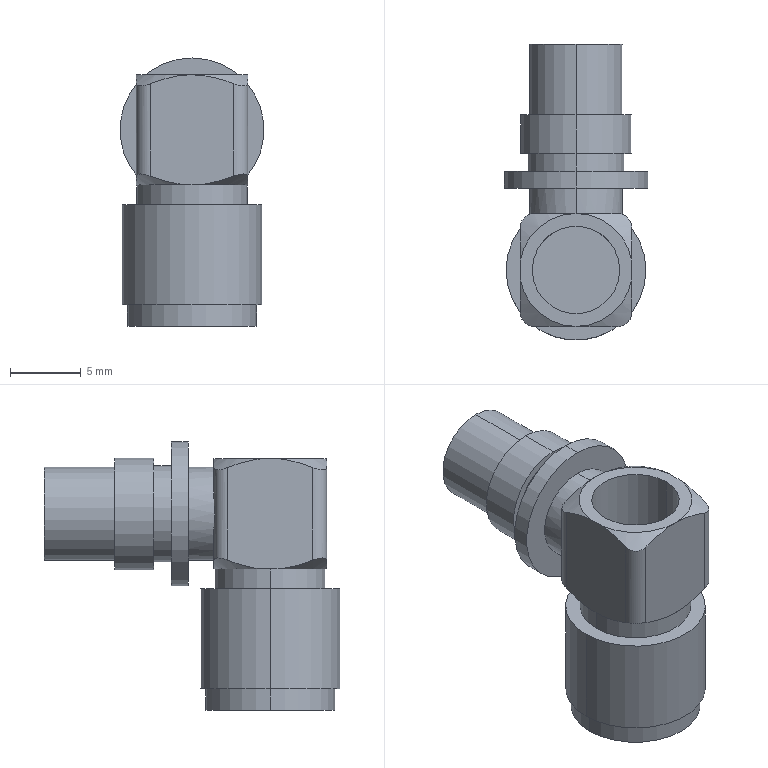Part | SolidWorks | features ICE 3, Revolution 2, Extrusion 1, Fillet 1, MirrorPattern 1, RevCut 1 | 1 solid | 57 faces | box 10.2 x 20.95 x 19 mm | volume 1460 mm3 | cylinder 28 | plane 17 | cone 12 | commonest cylinder face diameters 2 x4 6.6 x4 0.941 x2 5.6 x2 6.2 x2 6.8 x2